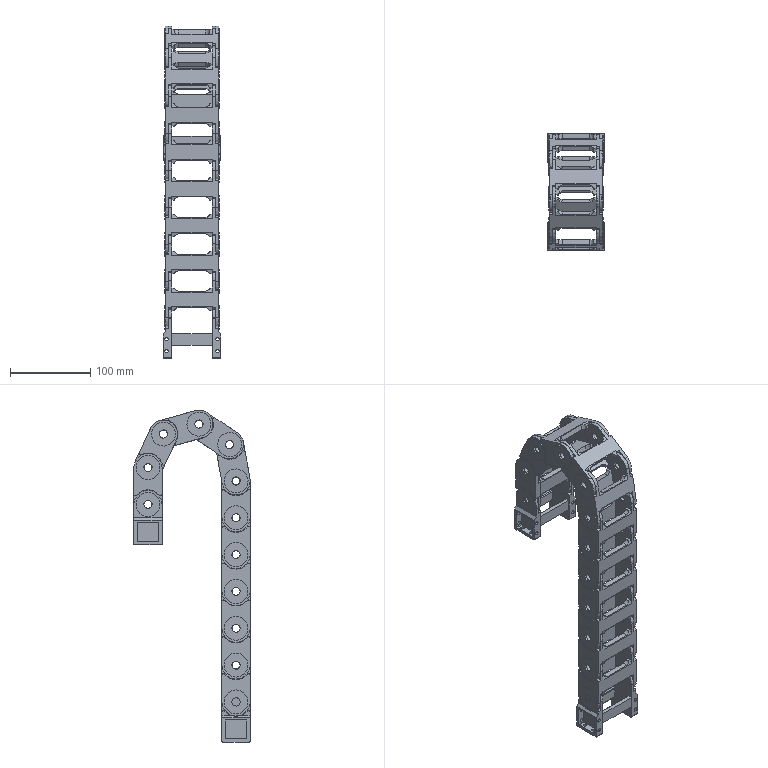Part | SolidWorks | 13 solids | 2961 faces | box 72.4 x 145.352 x 414.628 mm | volume 469160 mm3 | cylinder 1609 | plane 1352 | commonest cylinder face diameters 2 x482 4.24 x132 18.2 x96 32.34 x92 10 x88 13.7 x88